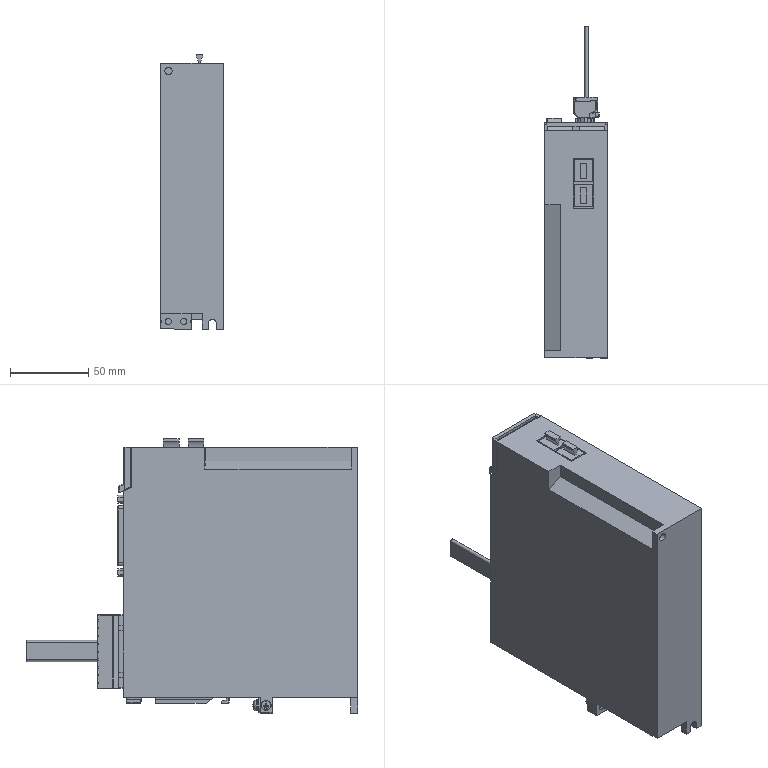Part | STEP file | 5 solids | 1381 faces | box 40 x 212 x 175.4 mm | volume 959953 mm3 | plane 909 | cylinder 387 | sphere 26 | spline 26 | cone 22 | torus 11 | commonest cylinder face diameters 1 x130 0.6 x104 0.4 x35 4.3 x18 4 x14 3.6 x13